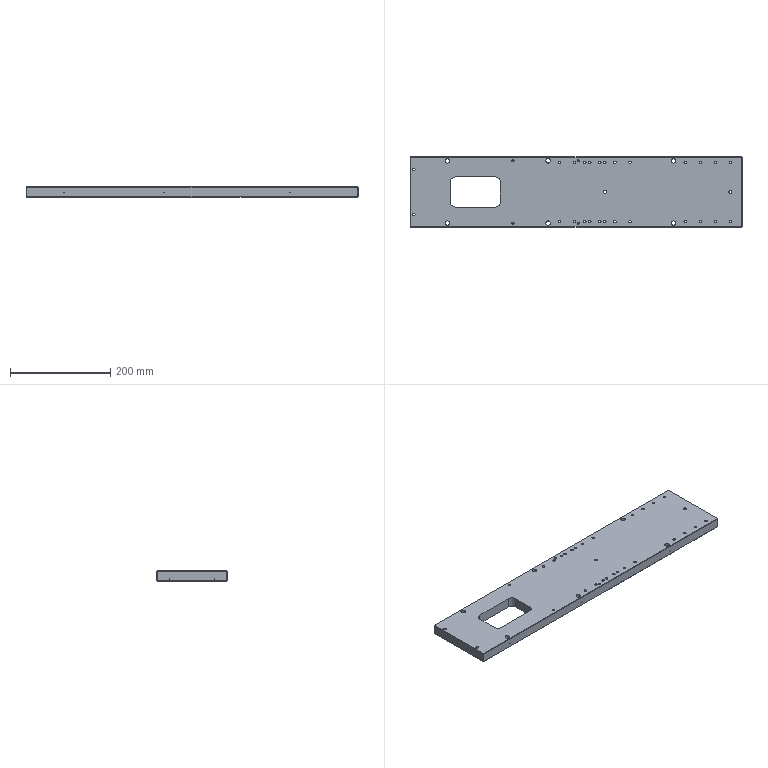Part | SolidWorks | features HoleWzd 4, Cut 3, ICE 2, Chamfer 1, Extrusion 1, Fillet 1, LibraryFeature 1 | 1 solid | 138 faces | box 661 x 140 x 20 mm | volume 1704232 mm3 | cylinder 96 | plane 38 | cone 4 | commonest cylinder face diameters 5 x48 9 x12 15 x12 4.2 x8 5.5 x4 6 x4